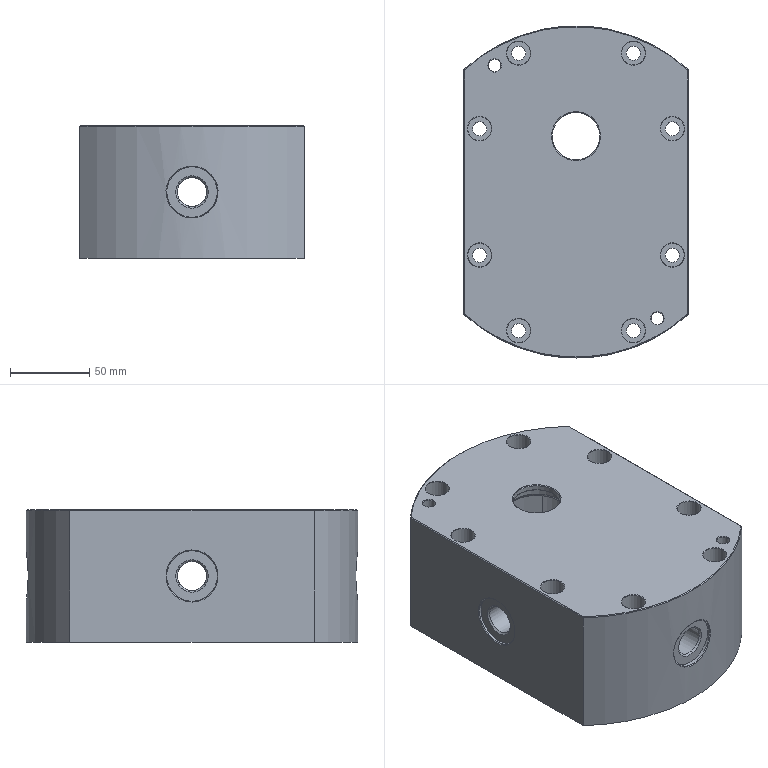NC program | NX | posted with a generic post | part box 142 x 210 x 84 mm
Lines 1 to 686 of 1634:
N10 G17 G21 G94 G90
(HOLE_MILLING_COPY_COPY , TOOL : D10)
N12 T10 M6
N14 G54
N16 G17 G0 G90 X-87.769 Y36.355 B0. C0. S3000 M3
N18 G43 Z30. H10
N20 Z0.5
N22 G94 G3 X-89.019 Y35.105 R1.25 F2200.
N24 X-87.769 Y33.855 R1.25
N26 X-87.769 Y33.855 Z0.28 I0. J2.5
N28 X-87.769 Y33.855 Z0.06 I0. J2.5
N30 X-87.769 Y33.855 Z-0.16 I0. J2.5
N32 X-87.769 Y33.855 Z-0.38 I0. J2.5
N34 X-87.769 Y33.855 Z-0.6 I0. J2.5
N36 X-87.769 Y33.855 Z-0.82 I0. J2.5
N38 X-87.769 Y33.855 Z-1.04 I0. J2.5
N40 X-87.769 Y33.855 Z-1.26 I0. J2.5
N42 X-87.769 Y33.855 Z-1.48 I0. J2.5
N44 X-87.769 Y33.855 Z-1.7 I0. J2.5
N46 X-87.769 Y33.855 Z-1.92 I0. J2.5
N48 X-87.769 Y33.855 Z-2.14 I0. J2.5
N50 X-87.769 Y33.855 Z-2.36 I0. J2.5
N52 X-87.769 Y33.855 Z-2.58 I0. J2.5
N54 X-87.769 Y33.855 Z-2.8 I0. J2.5
N56 X-87.769 Y33.855 Z-3.02 I0. J2.5
N58 X-87.769 Y33.855 Z-3.24 I0. J2.5
N60 X-87.769 Y33.855 Z-3.46 I0. J2.5
N62 X-87.769 Y33.855 Z-3.68 I0. J2.5
N64 X-87.769 Y33.855 Z-3.9 I0. J2.5
N66 X-87.769 Y33.855 Z-4.12 I0. J2.5
N68 X-87.769 Y33.855 Z-4.34 I0. J2.5
N70 X-87.769 Y33.855 Z-4.56 I0. J2.5
N72 X-87.769 Y33.855 Z-4.78 I0. J2.5
N74 X-87.769 Y33.855 Z-5. I0. J2.5
N76 X-87.769 Y33.855 Z-5.22 I0. J2.5
N78 X-87.769 Y33.855 Z-5.44 I0. J2.5
N80 X-87.769 Y33.855 Z-5.66 I0. J2.5
N82 X-87.769 Y33.855 Z-5.88 I0. J2.5
N84 X-87.769 Y33.855 Z-6.1 I0. J2.5
N86 X-87.769 Y33.855 Z-6.32 I0. J2.5
N88 X-87.769 Y33.855 Z-6.54 I0. J2.5
N90 X-87.769 Y33.855 Z-6.76 I0. J2.5
N92 X-87.769 Y33.855 Z-6.98 I0. J2.5
N94 X-87.769 Y33.855 Z-7.2 I0. J2.5
N96 X-87.769 Y33.855 Z-7.42 I0. J2.5
N98 X-87.769 Y33.855 Z-7.64 I0. J2.5
N100 X-87.769 Y33.855 Z-7.86 I0. J2.5
N102 X-87.769 Y33.855 Z-8.08 I0. J2.5
N104 X-87.769 Y33.855 Z-8.3 I0. J2.5
N106 X-87.769 Y33.855 Z-8.52 I0. J2.5
N108 X-87.769 Y33.855 Z-8.74 I0. J2.5
N110 X-87.769 Y33.855 Z-8.96 I0. J2.5
N112 X-87.769 Y33.855 Z-9.18 I0. J2.5
N114 X-87.769 Y33.855 Z-9.4 I0. J2.5
N116 X-87.769 Y33.855 Z-9.62 I0. J2.5
N118 X-87.769 Y33.855 Z-9.84 I0. J2.5
N120 X-87.769 Y33.855 Z-10.06 I0. J2.5
N122 X-87.769 Y33.855 Z-10.28 I0. J2.5
N124 X-87.769 Y33.855 Z-10.5 I0. J2.5
N126 X-87.769 Y33.855 Z-10.72 I0. J2.5
N128 X-87.769 Y33.855 Z-10.94 I0. J2.5
N130 X-87.769 Y33.855 Z-11.16 I0. J2.5
N132 X-87.769 Y33.855 Z-11.38 I0. J2.5
N134 X-87.769 Y33.855 Z-11.6 I0. J2.5
N136 X-87.769 Y33.855 Z-11.82 I0. J2.5
N138 X-87.769 Y33.855 Z-12.04 I0. J2.5
N140 X-87.769 Y33.855 Z-12.26 I0. J2.5
N142 X-87.769 Y33.855 Z-12.48 I0. J2.5
N144 X-87.769 Y33.855 Z-12.7 I0. J2.5
N146 X-87.769 Y33.855 Z-12.92 I0. J2.5
N148 X-87.769 Y33.855 Z-13.14 I0. J2.5
N150 X-87.769 Y33.855 Z-13.36 I0. J2.5
N152 X-87.769 Y33.855 Z-13.58 I0. J2.5
N154 X-87.769 Y33.855 Z-13.8 I0. J2.5
N156 X-87.769 Y33.855 Z-14.02 I0. J2.5
N158 X-87.769 Y33.855 Z-14.24 I0. J2.5
N160 X-87.769 Y33.855 Z-14.46 I0. J2.5
N162 X-87.769 Y33.855 Z-14.68 I0. J2.5
N164 X-87.769 Y33.855 Z-14.9 I0. J2.5
N166 X-87.769 Y33.855 Z-15.12 I0. J2.5
N168 X-87.769 Y33.855 Z-15.34 I0. J2.5
N170 X-87.769 Y33.855 Z-15.56 I0. J2.5
N172 X-87.769 Y33.855 Z-15.78 I0. J2.5
N174 X-87.769 Y33.855 Z-16. I0. J2.5
N176 X-87.769 Y33.855 Z-16.22 I0. J2.5
N178 X-87.769 Y33.855 Z-16.44 I0. J2.5
N180 X-87.769 Y33.855 Z-16.66 I0. J2.5
N182 X-87.769 Y33.855 Z-16.88 I0. J2.5
N184 X-87.769 Y33.855 Z-17.1 I0. J2.5
N186 X-87.769 Y33.855 Z-17.32 I0. J2.5
N188 X-87.769 Y33.855 Z-17.54 I0. J2.5
N190 X-87.769 Y33.855 Z-17.76 I0. J2.5
N192 X-87.769 Y33.855 Z-17.98 I0. J2.5
N194 X-87.769 Y33.855 Z-18.2 I0. J2.5
N196 X-87.769 Y33.855 Z-18.42 I0. J2.5
N198 X-87.769 Y33.855 Z-18.64 I0. J2.5
N200 X-87.769 Y33.855 Z-18.86 I0. J2.5
N202 X-87.769 Y33.855 Z-19.08 I0. J2.5
N204 X-87.769 Y33.855 Z-19.3 I0. J2.5
N206 X-87.769 Y33.855 Z-19.52 I0. J2.5
N208 X-87.769 Y33.855 Z-19.74 I0. J2.5
N210 X-87.769 Y33.855 Z-19.96 I0. J2.5
N212 X-87.769 Y33.855 Z-20.18 I0. J2.5
N214 X-87.769 Y33.855 Z-20.4 I0. J2.5
N216 X-87.769 Y33.855 Z-20.62 I0. J2.5
N218 X-87.769 Y33.855 Z-20.84 I0. J2.5
N220 X-87.769 Y33.855 Z-21.06 I0. J2.5
N222 X-87.769 Y33.855 Z-21.28 I0. J2.5
N224 X-87.769 Y33.855 Z-21.5 I0. J2.5
N226 X-87.769 Y33.855 Z-21.72 I0. J2.5
N228 X-87.769 Y33.855 Z-21.94 I0. J2.5
N230 X-87.769 Y33.855 Z-22.16 I0. J2.5
N232 X-87.769 Y33.855 Z-22.38 I0. J2.5
N234 X-87.769 Y33.855 Z-22.6 I0. J2.5
N236 X-87.769 Y33.855 Z-22.82 I0. J2.5
N238 X-87.769 Y33.855 Z-23.04 I0. J2.5
N240 X-87.769 Y33.855 Z-23.26 I0. J2.5
N242 X-87.769 Y33.855 Z-23.48 I0. J2.5
N244 X-87.769 Y33.855 Z-23.7 I0. J2.5
N246 X-87.769 Y33.855 Z-23.92 I0. J2.5
N248 X-87.769 Y33.855 Z-24.14 I0. J2.5
N250 X-87.769 Y33.855 Z-24.36 I0. J2.5
N252 X-87.769 Y33.855 Z-24.58 I0. J2.5
N254 X-87.769 Y33.855 Z-24.8 I0. J2.5
N256 X-87.769 Y33.855 Z-25.02 I0. J2.5
N258 X-87.769 Y33.855 Z-25.24 I0. J2.5
N260 X-87.769 Y33.855 Z-25.46 I0. J2.5
N262 X-87.769 Y33.855 Z-25.68 I0. J2.5
N264 X-87.769 Y33.855 Z-25.9 I0. J2.5
N266 X-87.769 Y33.855 Z-26.12 I0. J2.5
N268 X-87.769 Y33.855 Z-26.34 I0. J2.5
N270 X-87.769 Y33.855 Z-26.56 I0. J2.5
N272 X-87.769 Y33.855 Z-26.78 I0. J2.5
N274 X-87.769 Y33.855 Z-27. I0. J2.5
N276 X-87.769 Y33.855 Z-27.22 I0. J2.5
N278 X-87.769 Y33.855 Z-27.44 I0. J2.5
N280 X-87.769 Y33.855 Z-27.66 I0. J2.5
N282 X-87.769 Y33.855 Z-27.88 I0. J2.5
N284 X-87.769 Y33.855 Z-28.1 I0. J2.5
N286 X-87.769 Y33.855 Z-28.32 I0. J2.5
N288 X-87.769 Y33.855 Z-28.54 I0. J2.5
N290 X-87.769 Y33.855 Z-28.76 I0. J2.5
N292 X-87.769 Y33.855 Z-28.98 I0. J2.5
N294 X-87.769 Y33.855 Z-29.2 I0. J2.5
N296 X-87.769 Y33.855 Z-29.42 I0. J2.5
N298 X-87.769 Y33.855 Z-29.64 I0. J2.5
N300 X-87.769 Y33.855 Z-29.86 I0. J2.5
N302 X-87.769 Y33.855 Z-30.08 I0. J2.5
N304 X-87.769 Y33.855 Z-30.3 I0. J2.5
N306 X-87.769 Y33.855 Z-30.52 I0. J2.5
N308 X-87.769 Y33.855 Z-30.74 I0. J2.5
N310 X-87.769 Y33.855 Z-30.96 I0. J2.5
N312 X-87.769 Y33.855 Z-31.18 I0. J2.5
N314 X-87.769 Y33.855 Z-31.4 I0. J2.5
N316 X-87.769 Y33.855 Z-31.62 I0. J2.5
N318 X-87.769 Y33.855 Z-31.84 I0. J2.5
N320 X-87.769 Y33.855 Z-32.06 I0. J2.5
N322 X-87.769 Y33.855 Z-32.28 I0. J2.5
N324 X-87.769 Y33.855 Z-32.5 I0. J2.5
N326 X-87.769 Y33.855 Z-32.72 I0. J2.5
N328 X-87.769 Y33.855 Z-32.94 I0. J2.5
N330 X-87.769 Y33.855 Z-33.16 I0. J2.5
N332 X-87.769 Y33.855 Z-33.38 I0. J2.5
N334 X-87.769 Y33.855 Z-33.6 I0. J2.5
N336 X-87.769 Y33.855 Z-33.82 I0. J2.5
N338 X-87.769 Y33.855 Z-34.04 I0. J2.5
N340 X-87.769 Y33.855 Z-34.26 I0. J2.5
N342 X-87.769 Y33.855 Z-34.48 I0. J2.5
N344 X-87.769 Y33.855 Z-34.7 I0. J2.5
N346 X-87.769 Y33.855 Z-34.92 I0. J2.5
N348 X-85.879 Y37.992 Z-35. R2.5
N350 X-89.406 Y38.244 R2.5
N352 X-85.879 Y37.992 R-2.5
N354 X-87.642 Y38.118 R1.25
N356 X-87.769 Y36.355 R1.25
N358 G0 Z30.
N360 X-40. Y61.
N362 Z0.5
N364 G3 X-41.25 Y59.75 R1.25
N366 X-40. Y58.5 R1.25
N368 X-40. Y58.5 Z0.28 I0. J2.5
N370 X-40. Y58.5 Z0.06 I0. J2.5
N372 X-40. Y58.5 Z-0.16 I0. J2.5
N374 X-40. Y58.5 Z-0.38 I0. J2.5
N376 X-40. Y58.5 Z-0.6 I0. J2.5
N378 X-40. Y58.5 Z-0.82 I0. J2.5
N380 X-40. Y58.5 Z-1.04 I0. J2.5
N382 X-40. Y58.5 Z-1.26 I0. J2.5
N384 X-40. Y58.5 Z-1.48 I0. J2.5
N386 X-40. Y58.5 Z-1.7 I0. J2.5
N388 X-40. Y58.5 Z-1.92 I0. J2.5
N390 X-40. Y58.5 Z-2.14 I0. J2.5
N392 X-40. Y58.5 Z-2.36 I0. J2.5
N394 X-40. Y58.5 Z-2.58 I0. J2.5
N396 X-40. Y58.5 Z-2.8 I0. J2.5
N398 X-40. Y58.5 Z-3.02 I0. J2.5
N400 X-40. Y58.5 Z-3.24 I0. J2.5
N402 X-40. Y58.5 Z-3.46 I0. J2.5
N404 X-40. Y58.5 Z-3.68 I0. J2.5
N406 X-40. Y58.5 Z-3.9 I0. J2.5
N408 X-40. Y58.5 Z-4.12 I0. J2.5
N410 X-40. Y58.5 Z-4.34 I0. J2.5
N412 X-40. Y58.5 Z-4.56 I0. J2.5
N414 X-40. Y58.5 Z-4.78 I0. J2.5
N416 X-40. Y58.5 Z-5. I0. J2.5
N418 X-40. Y58.5 Z-5.22 I0. J2.5
N420 X-40. Y58.5 Z-5.44 I0. J2.5
N422 X-40. Y58.5 Z-5.66 I0. J2.5
N424 X-40. Y58.5 Z-5.88 I0. J2.5
N426 X-40. Y58.5 Z-6.1 I0. J2.5
N428 X-40. Y58.5 Z-6.32 I0. J2.5
N430 X-40. Y58.5 Z-6.54 I0. J2.5
N432 X-40. Y58.5 Z-6.76 I0. J2.5
N434 X-40. Y58.5 Z-6.98 I0. J2.5
N436 X-40. Y58.5 Z-7.2 I0. J2.5
N438 X-40. Y58.5 Z-7.42 I0. J2.5
N440 X-40. Y58.5 Z-7.64 I0. J2.5
N442 X-40. Y58.5 Z-7.86 I0. J2.5
N444 X-40. Y58.5 Z-8.08 I0. J2.5
N446 X-40. Y58.5 Z-8.3 I0. J2.5
N448 X-40. Y58.5 Z-8.52 I0. J2.5
N450 X-40. Y58.5 Z-8.74 I0. J2.5
N452 X-40. Y58.5 Z-8.96 I0. J2.5
N454 X-40. Y58.5 Z-9.18 I0. J2.5
N456 X-40. Y58.5 Z-9.4 I0. J2.5
N458 X-40. Y58.5 Z-9.62 I0. J2.5
N460 X-40. Y58.5 Z-9.84 I0. J2.5
N462 X-40. Y58.5 Z-10.06 I0. J2.5
N464 X-40. Y58.5 Z-10.28 I0. J2.5
N466 X-40. Y58.5 Z-10.5 I0. J2.5
N468 X-40. Y58.5 Z-10.72 I0. J2.5
N470 X-40. Y58.5 Z-10.94 I0. J2.5
N472 X-40. Y58.5 Z-11.16 I0. J2.5
N474 X-40. Y58.5 Z-11.38 I0. J2.5
N476 X-40. Y58.5 Z-11.6 I0. J2.5
N478 X-40. Y58.5 Z-11.82 I0. J2.5
N480 X-40. Y58.5 Z-12.04 I0. J2.5
N482 X-40. Y58.5 Z-12.26 I0. J2.5
N484 X-40. Y58.5 Z-12.48 I0. J2.5
N486 X-40. Y58.5 Z-12.7 I0. J2.5
N488 X-40. Y58.5 Z-12.92 I0. J2.5
N490 X-40. Y58.5 Z-13.14 I0. J2.5
N492 X-40. Y58.5 Z-13.36 I0. J2.5
N494 X-40. Y58.5 Z-13.58 I0. J2.5
N496 X-40. Y58.5 Z-13.8 I0. J2.5
N498 X-40. Y58.5 Z-14.02 I0. J2.5
N500 X-40. Y58.5 Z-14.24 I0. J2.5
N502 X-40. Y58.5 Z-14.46 I0. J2.5
N504 X-40. Y58.5 Z-14.68 I0. J2.5
N506 X-40. Y58.5 Z-14.9 I0. J2.5
N508 X-40. Y58.5 Z-15.12 I0. J2.5
N510 X-40. Y58.5 Z-15.34 I0. J2.5
N512 X-40. Y58.5 Z-15.56 I0. J2.5
N514 X-40. Y58.5 Z-15.78 I0. J2.5
N516 X-40. Y58.5 Z-16. I0. J2.5
N518 X-40. Y58.5 Z-16.22 I0. J2.5
N520 X-40. Y58.5 Z-16.44 I0. J2.5
N522 X-40. Y58.5 Z-16.66 I0. J2.5
N524 X-40. Y58.5 Z-16.88 I0. J2.5
N526 X-40. Y58.5 Z-17.1 I0. J2.5
N528 X-40. Y58.5 Z-17.32 I0. J2.5
N530 X-40. Y58.5 Z-17.54 I0. J2.5
N532 X-40. Y58.5 Z-17.76 I0. J2.5
N534 X-40. Y58.5 Z-17.98 I0. J2.5
N536 X-40. Y58.5 Z-18.2 I0. J2.5
N538 X-40. Y58.5 Z-18.42 I0. J2.5
N540 X-40. Y58.5 Z-18.64 I0. J2.5
N542 X-40. Y58.5 Z-18.86 I0. J2.5
N544 X-40. Y58.5 Z-19.08 I0. J2.5
N546 X-40. Y58.5 Z-19.3 I0. J2.5
N548 X-40. Y58.5 Z-19.52 I0. J2.5
N550 X-40. Y58.5 Z-19.74 I0. J2.5
N552 X-40. Y58.5 Z-19.96 I0. J2.5
N554 X-40. Y58.5 Z-20.18 I0. J2.5
N556 X-40. Y58.5 Z-20.4 I0. J2.5
N558 X-40. Y58.5 Z-20.62 I0. J2.5
N560 X-40. Y58.5 Z-20.84 I0. J2.5
N562 X-40. Y58.5 Z-21.06 I0. J2.5
N564 X-40. Y58.5 Z-21.28 I0. J2.5
N566 X-40. Y58.5 Z-21.5 I0. J2.5
N568 X-40. Y58.5 Z-21.72 I0. J2.5
N570 X-40. Y58.5 Z-21.94 I0. J2.5
N572 X-40. Y58.5 Z-22.16 I0. J2.5
N574 X-40. Y58.5 Z-22.38 I0. J2.5
N576 X-40. Y58.5 Z-22.6 I0. J2.5
N578 X-40. Y58.5 Z-22.82 I0. J2.5
N580 X-40. Y58.5 Z-23.04 I0. J2.5
N582 X-40. Y58.5 Z-23.26 I0. J2.5
N584 X-40. Y58.5 Z-23.48 I0. J2.5
N586 X-40. Y58.5 Z-23.7 I0. J2.5
N588 X-40. Y58.5 Z-23.92 I0. J2.5
N590 X-40. Y58.5 Z-24.14 I0. J2.5
N592 X-40. Y58.5 Z-24.36 I0. J2.5
N594 X-40. Y58.5 Z-24.58 I0. J2.5
N596 X-40. Y58.5 Z-24.8 I0. J2.5
N598 X-40. Y58.5 Z-25.02 I0. J2.5
N600 X-40. Y58.5 Z-25.24 I0. J2.5
N602 X-40. Y58.5 Z-25.46 I0. J2.5
N604 X-40. Y58.5 Z-25.68 I0. J2.5
N606 X-40. Y58.5 Z-25.9 I0. J2.5
N608 X-40. Y58.5 Z-26.12 I0. J2.5
N610 X-40. Y58.5 Z-26.34 I0. J2.5
N612 X-40. Y58.5 Z-26.56 I0. J2.5
N614 X-40. Y58.5 Z-26.78 I0. J2.5
N616 X-40. Y58.5 Z-27. I0. J2.5
N618 X-40. Y58.5 Z-27.22 I0. J2.5
N620 X-40. Y58.5 Z-27.44 I0. J2.5
N622 X-40. Y58.5 Z-27.66 I0. J2.5
N624 X-40. Y58.5 Z-27.88 I0. J2.5
N626 X-40. Y58.5 Z-28.1 I0. J2.5
N628 X-40. Y58.5 Z-28.32 I0. J2.5
N630 X-40. Y58.5 Z-28.54 I0. J2.5
N632 X-40. Y58.5 Z-28.76 I0. J2.5
N634 X-40. Y58.5 Z-28.98 I0. J2.5
N636 X-40. Y58.5 Z-29.2 I0. J2.5
N638 X-40. Y58.5 Z-29.42 I0. J2.5
N640 X-40. Y58.5 Z-29.64 I0. J2.5
N642 X-40. Y58.5 Z-29.86 I0. J2.5
N644 X-40. Y58.5 Z-30.08 I0. J2.5
N646 X-40. Y58.5 Z-30.3 I0. J2.5
N648 X-40. Y58.5 Z-30.52 I0. J2.5
N650 X-40. Y58.5 Z-30.74 I0. J2.5
N652 X-40. Y58.5 Z-30.96 I0. J2.5
N654 X-40. Y58.5 Z-31.18 I0. J2.5
N656 X-40. Y58.5 Z-31.4 I0. J2.5
N658 X-40. Y58.5 Z-31.62 I0. J2.5
N660 X-40. Y58.5 Z-31.84 I0. J2.5
N662 X-40. Y58.5 Z-32.06 I0. J2.5
N664 X-40. Y58.5 Z-32.28 I0. J2.5
N666 X-40. Y58.5 Z-32.5 I0. J2.5
N668 X-40. Y58.5 Z-32.72 I0. J2.5
N670 X-40. Y58.5 Z-32.94 I0. J2.5
N672 X-40. Y58.5 Z-33.16 I0. J2.5
N674 X-40. Y58.5 Z-33.38 I0. J2.5
N676 X-40. Y58.5 Z-33.6 I0. J2.5
N678 X-40. Y58.5 Z-33.82 I0. J2.5
N680 X-40. Y58.5 Z-34.04 I0. J2.5
N682 X-40. Y58.5 Z-34.26 I0. J2.5
N684 X-40. Y58.5 Z-34.48 I0. J2.5
N686 X-40. Y58.5 Z-34.7 I0. J2.5
N688 X-40. Y58.5 Z-34.92 I0. J2.5
N690 X-38.111 Y62.637 Z-35. R2.5
N692 X-41.637 Y62.889 R2.5
N694 X-38.111 Y62.637 R-2.5
N696 X-39.874 Y62.763 R1.25
N698 X-40. Y61. R1.25
N700 G0 Z30.
N702 X40.
N704 Z0.5
N706 G3 X38.75 Y59.75 R1.25
N708 X40. Y58.5 R1.25
N710 X40. Y58.5 Z0.28 I0. J2.5
N712 X40. Y58.5 Z0.06 I0. J2.5
N714 X40. Y58.5 Z-0.16 I0. J2.5
N716 X40. Y58.5 Z-0.38 I0. J2.5
N718 X40. Y58.5 Z-0.6 I0. J2.5
N720 X40. Y58.5 Z-0.82 I0. J2.5
N722 X40. Y58.5 Z-1.04 I0. J2.5
N724 X40. Y58.5 Z-1.26 I0. J2.5
N726 X40. Y58.5 Z-1.48 I0. J2.5
N728 X40. Y58.5 Z-1.7 I0. J2.5
N730 X40. Y58.5 Z-1.92 I0. J2.5
N732 X40. Y58.5 Z-2.14 I0. J2.5
N734 X40. Y58.5 Z-2.36 I0. J2.5
N736 X40. Y58.5 Z-2.58 I0. J2.5
N738 X40. Y58.5 Z-2.8 I0. J2.5
N740 X40. Y58.5 Z-3.02 I0. J2.5
N742 X40. Y58.5 Z-3.24 I0. J2.5
N744 X40. Y58.5 Z-3.46 I0. J2.5
N746 X40. Y58.5 Z-3.68 I0. J2.5
N748 X40. Y58.5 Z-3.9 I0. J2.5
N750 X40. Y58.5 Z-4.12 I0. J2.5
N752 X40. Y58.5 Z-4.34 I0. J2.5
N754 X40. Y58.5 Z-4.56 I0. J2.5
N756 X40. Y58.5 Z-4.78 I0. J2.5
N758 X40. Y58.5 Z-5. I0. J2.5
N760 X40. Y58.5 Z-5.22 I0. J2.5
N762 X40. Y58.5 Z-5.44 I0. J2.5
N764 X40. Y58.5 Z-5.66 I0. J2.5
N766 X40. Y58.5 Z-5.88 I0. J2.5
N768 X40. Y58.5 Z-6.1 I0. J2.5
N770 X40. Y58.5 Z-6.32 I0. J2.5
N772 X40. Y58.5 Z-6.54 I0. J2.5
N774 X40. Y58.5 Z-6.76 I0. J2.5
N776 X40. Y58.5 Z-6.98 I0. J2.5
N778 X40. Y58.5 Z-7.2 I0. J2.5
N780 X40. Y58.5 Z-7.42 I0. J2.5
N782 X40. Y58.5 Z-7.64 I0. J2.5
N784 X40. Y58.5 Z-7.86 I0. J2.5
N786 X40. Y58.5 Z-8.08 I0. J2.5
N788 X40. Y58.5 Z-8.3 I0. J2.5
N790 X40. Y58.5 Z-8.52 I0. J2.5
N792 X40. Y58.5 Z-8.74 I0. J2.5
N794 X40. Y58.5 Z-8.96 I0. J2.5
N796 X40. Y58.5 Z-9.18 I0. J2.5
N798 X40. Y58.5 Z-9.4 I0. J2.5
N800 X40. Y58.5 Z-9.62 I0. J2.5
N802 X40. Y58.5 Z-9.84 I0. J2.5
N804 X40. Y58.5 Z-10.06 I0. J2.5
N806 X40. Y58.5 Z-10.28 I0. J2.5
N808 X40. Y58.5 Z-10.5 I0. J2.5
N810 X40. Y58.5 Z-10.72 I0. J2.5
N812 X40. Y58.5 Z-10.94 I0. J2.5
N814 X40. Y58.5 Z-11.16 I0. J2.5
N816 X40. Y58.5 Z-11.38 I0. J2.5
N818 X40. Y58.5 Z-11.6 I0. J2.5
N820 X40. Y58.5 Z-11.82 I0. J2.5
N822 X40. Y58.5 Z-12.04 I0. J2.5
N824 X40. Y58.5 Z-12.26 I0. J2.5
N826 X40. Y58.5 Z-12.48 I0. J2.5
N828 X40. Y58.5 Z-12.7 I0. J2.5
N830 X40. Y58.5 Z-12.92 I0. J2.5
N832 X40. Y58.5 Z-13.14 I0. J2.5
N834 X40. Y58.5 Z-13.36 I0. J2.5
N836 X40. Y58.5 Z-13.58 I0. J2.5
N838 X40. Y58.5 Z-13.8 I0. J2.5
N840 X40. Y58.5 Z-14.02 I0. J2.5
N842 X40. Y58.5 Z-14.24 I0. J2.5
N844 X40. Y58.5 Z-14.46 I0. J2.5
N846 X40. Y58.5 Z-14.68 I0. J2.5
N848 X40. Y58.5 Z-14.9 I0. J2.5
N850 X40. Y58.5 Z-15.12 I0. J2.5
N852 X40. Y58.5 Z-15.34 I0. J2.5
N854 X40. Y58.5 Z-15.56 I0. J2.5
N856 X40. Y58.5 Z-15.78 I0. J2.5
N858 X40. Y58.5 Z-16. I0. J2.5
N860 X40. Y58.5 Z-16.22 I0. J2.5
N862 X40. Y58.5 Z-16.44 I0. J2.5
N864 X40. Y58.5 Z-16.66 I0. J2.5
N866 X40. Y58.5 Z-16.88 I0. J2.5
N868 X40. Y58.5 Z-17.1 I0. J2.5
N870 X40. Y58.5 Z-17.32 I0. J2.5
N872 X40. Y58.5 Z-17.54 I0. J2.5
N874 X40. Y58.5 Z-17.76 I0. J2.5
N876 X40. Y58.5 Z-17.98 I0. J2.5
N878 X40. Y58.5 Z-18.2 I0. J2.5
N880 X40. Y58.5 Z-18.42 I0. J2.5
N882 X40. Y58.5 Z-18.64 I0. J2.5
N884 X40. Y58.5 Z-18.86 I0. J2.5
N886 X40. Y58.5 Z-19.08 I0. J2.5
N888 X40. Y58.5 Z-19.3 I0. J2.5
N890 X40. Y58.5 Z-19.52 I0. J2.5
N892 X40. Y58.5 Z-19.74 I0. J2.5
N894 X40. Y58.5 Z-19.96 I0. J2.5
N896 X40. Y58.5 Z-20.18 I0. J2.5
N898 X40. Y58.5 Z-20.4 I0. J2.5
N900 X40. Y58.5 Z-20.62 I0. J2.5
N902 X40. Y58.5 Z-20.84 I0. J2.5
N904 X40. Y58.5 Z-21.06 I0. J2.5
N906 X40. Y58.5 Z-21.28 I0. J2.5
N908 X40. Y58.5 Z-21.5 I0. J2.5
N910 X40. Y58.5 Z-21.72 I0. J2.5
N912 X40. Y58.5 Z-21.94 I0. J2.5
N914 X40. Y58.5 Z-22.16 I0. J2.5
N916 X40. Y58.5 Z-22.38 I0. J2.5
N918 X40. Y58.5 Z-22.6 I0. J2.5
N920 X40. Y58.5 Z-22.82 I0. J2.5
N922 X40. Y58.5 Z-23.04 I0. J2.5
N924 X40. Y58.5 Z-23.26 I0. J2.5
N926 X40. Y58.5 Z-23.48 I0. J2.5
N928 X40. Y58.5 Z-23.7 I0. J2.5
N930 X40. Y58.5 Z-23.92 I0. J2.5
N932 X40. Y58.5 Z-24.14 I0. J2.5
N934 X40. Y58.5 Z-24.36 I0. J2.5
N936 X40. Y58.5 Z-24.58 I0. J2.5
N938 X40. Y58.5 Z-24.8 I0. J2.5
N940 X40. Y58.5 Z-25.02 I0. J2.5
N942 X40. Y58.5 Z-25.24 I0. J2.5
N944 X40. Y58.5 Z-25.46 I0. J2.5
N946 X40. Y58.5 Z-25.68 I0. J2.5
N948 X40. Y58.5 Z-25.9 I0. J2.5
N950 X40. Y58.5 Z-26.12 I0. J2.5
N952 X40. Y58.5 Z-26.34 I0. J2.5
N954 X40. Y58.5 Z-26.56 I0. J2.5
N956 X40. Y58.5 Z-26.78 I0. J2.5
N958 X40. Y58.5 Z-27. I0. J2.5
N960 X40. Y58.5 Z-27.22 I0. J2.5
N962 X40. Y58.5 Z-27.44 I0. J2.5
N964 X40. Y58.5 Z-27.66 I0. J2.5
N966 X40. Y58.5 Z-27.88 I0. J2.5
N968 X40. Y58.5 Z-28.1 I0. J2.5
N970 X40. Y58.5 Z-28.32 I0. J2.5
N972 X40. Y58.5 Z-28.54 I0. J2.5
N974 X40. Y58.5 Z-28.76 I0. J2.5
N976 X40. Y58.5 Z-28.98 I0. J2.5
N978 X40. Y58.5 Z-29.2 I0. J2.5
N980 X40. Y58.5 Z-29.42 I0. J2.5
N982 X40. Y58.5 Z-29.64 I0. J2.5
N984 X40. Y58.5 Z-29.86 I0. J2.5
N986 X40. Y58.5 Z-30.08 I0. J2.5
N988 X40. Y58.5 Z-30.3 I0. J2.5
N990 X40. Y58.5 Z-30.52 I0. J2.5
N992 X40. Y58.5 Z-30.74 I0. J2.5
N994 X40. Y58.5 Z-30.96 I0. J2.5
N996 X40. Y58.5 Z-31.18 I0. J2.5
N998 X40. Y58.5 Z-31.4 I0. J2.5
N1000 X40. Y58.5 Z-31.62 I0. J2.5
N1002 X40. Y58.5 Z-31.84 I0. J2.5
N1004 X40. Y58.5 Z-32.06 I0. J2.5
N1006 X40. Y58.5 Z-32.28 I0. J2.5
N1008 X40. Y58.5 Z-32.5 I0. J2.5
N1010 X40. Y58.5 Z-32.72 I0. J2.5
N1012 X40. Y58.5 Z-32.94 I0. J2.5
N1014 X40. Y58.5 Z-33.16 I0. J2.5
N1016 X40. Y58.5 Z-33.38 I0. J2.5
N1018 X40. Y58.5 Z-33.6 I0. J2.5
N1020 X40. Y58.5 Z-33.82 I0. J2.5
N1022 X40. Y58.5 Z-34.04 I0. J2.5
N1024 X40. Y58.5 Z-34.26 I0. J2.5
N1026 X40. Y58.5 Z-34.48 I0. J2.5
N1028 X40. Y58.5 Z-34.7 I0. J2.5
N1030 X40. Y58.5 Z-34.92 I0. J2.5
N1032 X41.889 Y62.637 Z-35. R2.5
N1034 X38.363 Y62.889 R2.5
N1036 X41.889 Y62.637 R-2.5
N1038 X40.126 Y62.763 R1.25
N1040 X40. Y61. R1.25
N1042 G0 Z30.
N1044 X87.769 Y36.355
N1046 Z0.5
N1048 G3 X86.519 Y35.105 R1.25
N1050 X87.769 Y33.855 R1.25
N1052 X87.769 Y33.855 Z0.28 I0. J2.5
N1054 X87.769 Y33.855 Z0.06 I0. J2.5
N1056 X87.769 Y33.855 Z-0.16 I0. J2.5
N1058 X87.769 Y33.855 Z-0.38 I0. J2.5
N1060 X87.769 Y33.855 Z-0.6 I0. J2.5
N1062 X87.769 Y33.855 Z-0.82 I0. J2.5
N1064 X87.769 Y33.855 Z-1.04 I0. J2.5
N1066 X87.769 Y33.855 Z-1.26 I0. J2.5
N1068 X87.769 Y33.855 Z-1.48 I0. J2.5
N1070 X87.769 Y33.855 Z-1.7 I0. J2.5
N1072 X87.769 Y33.855 Z-1.92 I0. J2.5
N1074 X87.769 Y33.855 Z-2.14 I0. J2.5
N1076 X87.769 Y33.855 Z-2.36 I0. J2.5
N1078 X87.769 Y33.855 Z-2.58 I0. J2.5
N1080 X87.769 Y33.855 Z-2.8 I0. J2.5
N1082 X87.769 Y33.855 Z-3.02 I0. J2.5
N1084 X87.769 Y33.855 Z-3.24 I0. J2.5
N1086 X87.769 Y33.855 Z-3.46 I0. J2.5
N1088 X87.769 Y33.855 Z-3.68 I0. J2.5
N1090 X87.769 Y33.855 Z-3.9 I0. J2.5
N1092 X87.769 Y33.855 Z-4.12 I0. J2.5
N1094 X87.769 Y33.855 Z-4.34 I0. J2.5
N1096 X87.769 Y33.855 Z-4.56 I0. J2.5
N1098 X87.769 Y33.855 Z-4.78 I0. J2.5
N1100 X87.769 Y33.855 Z-5. I0. J2.5
N1102 X87.769 Y33.855 Z-5.22 I0. J2.5
N1104 X87.769 Y33.855 Z-5.44 I0. J2.5
N1106 X87.769 Y33.855 Z-5.66 I0. J2.5
N1108 X87.769 Y33.855 Z-5.88 I0. J2.5
N1110 X87.769 Y33.855 Z-6.1 I0. J2.5
N1112 X87.769 Y33.855 Z-6.32 I0. J2.5
N1114 X87.769 Y33.855 Z-6.54 I0. J2.5
N1116 X87.769 Y33.855 Z-6.76 I0. J2.5
N1118 X87.769 Y33.855 Z-6.98 I0. J2.5
N1120 X87.769 Y33.855 Z-7.2 I0. J2.5
N1122 X87.769 Y33.855 Z-7.42 I0. J2.5
N1124 X87.769 Y33.855 Z-7.64 I0. J2.5
N1126 X87.769 Y33.855 Z-7.86 I0. J2.5
N1128 X87.769 Y33.855 Z-8.08 I0. J2.5
N1130 X87.769 Y33.855 Z-8.3 I0. J2.5
N1132 X87.769 Y33.855 Z-8.52 I0. J2.5
N1134 X87.769 Y33.855 Z-8.74 I0. J2.5
N1136 X87.769 Y33.855 Z-8.96 I0. J2.5
N1138 X87.769 Y33.855 Z-9.18 I0. J2.5
N1140 X87.769 Y33.855 Z-9.4 I0. J2.5
N1142 X87.769 Y33.855 Z-9.62 I0. J2.5
N1144 X87.769 Y33.855 Z-9.84 I0. J2.5
N1146 X87.769 Y33.855 Z-10.06 I0. J2.5
N1148 X87.769 Y33.855 Z-10.28 I0. J2.5
N1150 X87.769 Y33.855 Z-10.5 I0. J2.5
N1152 X87.769 Y33.855 Z-10.72 I0. J2.5
N1154 X87.769 Y33.855 Z-10.94 I0. J2.5
N1156 X87.769 Y33.855 Z-11.16 I0. J2.5
N1158 X87.769 Y33.855 Z-11.38 I0. J2.5
N1160 X87.769 Y33.855 Z-11.6 I0. J2.5
N1162 X87.769 Y33.855 Z-11.82 I0. J2.5
N1164 X87.769 Y33.855 Z-12.04 I0. J2.5
N1166 X87.769 Y33.855 Z-12.26 I0. J2.5
N1168 X87.769 Y33.855 Z-12.48 I0. J2.5
N1170 X87.769 Y33.855 Z-12.7 I0. J2.5
N1172 X87.769 Y33.855 Z-12.92 I0. J2.5
N1174 X87.769 Y33.855 Z-13.14 I0. J2.5
N1176 X87.769 Y33.855 Z-13.36 I0. J2.5
N1178 X87.769 Y33.855 Z-13.58 I0. J2.5
N1180 X87.769 Y33.855 Z-13.8 I0. J2.5
N1182 X87.769 Y33.855 Z-14.02 I0. J2.5
N1184 X87.769 Y33.855 Z-14.24 I0. J2.5
N1186 X87.769 Y33.855 Z-14.46 I0. J2.5
N1188 X87.769 Y33.855 Z-14.68 I0. J2.5
N1190 X87.769 Y33.855 Z-14.9 I0. J2.5
N1192 X87.769 Y33.855 Z-15.12 I0. J2.5
N1194 X87.769 Y33.855 Z-15.34 I0. J2.5
N1196 X87.769 Y33.855 Z-15.56 I0. J2.5
N1198 X87.769 Y33.855 Z-15.78 I0. J2.5
N1200 X87.769 Y33.855 Z-16. I0. J2.5
N1202 X87.769 Y33.855 Z-16.22 I0. J2.5
N1204 X87.769 Y33.855 Z-16.44 I0. J2.5
N1206 X87.769 Y33.855 Z-16.66 I0. J2.5
N1208 X87.769 Y33.855 Z-16.88 I0. J2.5
N1210 X87.769 Y33.855 Z-17.1 I0. J2.5
N1212 X87.769 Y33.855 Z-17.32 I0. J2.5
N1214 X87.769 Y33.855 Z-17.54 I0. J2.5
N1216 X87.769 Y33.855 Z-17.76 I0. J2.5
N1218 X87.769 Y33.855 Z-17.98 I0. J2.5
N1220 X87.769 Y33.855 Z-18.2 I0. J2.5
N1222 X87.769 Y33.855 Z-18.42 I0. J2.5
N1224 X87.769 Y33.855 Z-18.64 I0. J2.5
N1226 X87.769 Y33.855 Z-18.86 I0. J2.5
N1228 X87.769 Y33.855 Z-19.08 I0. J2.5
N1230 X87.769 Y33.855 Z-19.3 I0. J2.5
N1232 X87.769 Y33.855 Z-19.52 I0. J2.5
N1234 X87.769 Y33.855 Z-19.74 I0. J2.5
N1236 X87.769 Y33.855 Z-19.96 I0. J2.5
N1238 X87.769 Y33.855 Z-20.18 I0. J2.5
N1240 X87.769 Y33.855 Z-20.4 I0. J2.5
N1242 X87.769 Y33.855 Z-20.62 I0. J2.5
N1244 X87.769 Y33.855 Z-20.84 I0. J2.5
N1246 X87.769 Y33.855 Z-21.06 I0. J2.5
N1248 X87.769 Y33.855 Z-21.28 I0. J2.5
N1250 X87.769 Y33.855 Z-21.5 I0. J2.5
N1252 X87.769 Y33.855 Z-21.72 I0. J2.5
N1254 X87.769 Y33.855 Z-21.94 I0. J2.5
N1256 X87.769 Y33.855 Z-22.16 I0. J2.5
N1258 X87.769 Y33.855 Z-22.38 I0. J2.5
N1260 X87.769 Y33.855 Z-22.6 I0. J2.5
N1262 X87.769 Y33.855 Z-22.82 I0. J2.5
N1264 X87.769 Y33.855 Z-23.04 I0. J2.5
N1266 X87.769 Y33.855 Z-23.26 I0. J2.5
N1268 X87.769 Y33.855 Z-23.48 I0. J2.5
N1270 X87.769 Y33.855 Z-23.7 I0. J2.5
N1272 X87.769 Y33.855 Z-23.92 I0. J2.5
N1274 X87.769 Y33.855 Z-24.14 I0. J2.5
N1276 X87.769 Y33.855 Z-24.36 I0. J2.5
N1278 X87.769 Y33.855 Z-24.58 I0. J2.5
N1280 X87.769 Y33.855 Z-24.8 I0. J2.5
N1282 X87.769 Y33.855 Z-25.02 I0. J2.5
N1284 X87.769 Y33.855 Z-25.24 I0. J2.5
N1286 X87.769 Y33.855 Z-25.46 I0. J2.5
N1288 X87.769 Y33.855 Z-25.68 I0. J2.5
N1290 X87.769 Y33.855 Z-25.9 I0. J2.5
N1292 X87.769 Y33.855 Z-26.12 I0. J2.5
N1294 X87.769 Y33.855 Z-26.34 I0. J2.5
N1296 X87.769 Y33.855 Z-26.56 I0. J2.5
N1298 X87.769 Y33.855 Z-26.78 I0. J2.5
N1300 X87.769 Y33.855 Z-27. I0. J2.5
N1302 X87.769 Y33.855 Z-27.22 I0. J2.5
N1304 X87.769 Y33.855 Z-27.44 I0. J2.5
N1306 X87.769 Y33.855 Z-27.66 I0. J2.5
N1308 X87.769 Y33.855 Z-27.88 I0. J2.5
N1310 X87.769 Y33.855 Z-28.1 I0. J2.5
N1312 X87.769 Y33.855 Z-28.32 I0. J2.5
N1314 X87.769 Y33.855 Z-28.54 I0. J2.5
N1316 X87.769 Y33.855 Z-28.76 I0. J2.5
N1318 X87.769 Y33.855 Z-28.98 I0. J2.5
N1320 X87.769 Y33.855 Z-29.2 I0. J2.5
N1322 X87.769 Y33.855 Z-29.42 I0. J2.5
N1324 X87.769 Y33.855 Z-29.64 I0. J2.5
N1326 X87.769 Y33.855 Z-29.86 I0. J2.5
N1328 X87.769 Y33.855 Z-30.08 I0. J2.5
N1330 X87.769 Y33.855 Z-30.3 I0. J2.5
N1332 X87.769 Y33.855 Z-30.52 I0. J2.5
N1334 X87.769 Y33.855 Z-30.74 I0. J2.5
N1336 X87.769 Y33.855 Z-30.96 I0. J2.5
N1338 X87.769 Y33.855 Z-31.18 I0. J2.5
N1340 X87.769 Y33.855 Z-31.4 I0. J2.5
N1342 X87.769 Y33.855 Z-31.62 I0. J2.5
N1344 X87.769 Y33.855 Z-31.84 I0. J2.5
N1346 X87.769 Y33.855 Z-32.06 I0. J2.5
N1348 X87.769 Y33.855 Z-32.28 I0. J2.5
N1350 X87.769 Y33.855 Z-32.5 I0. J2.5
N1352 X87.769 Y33.855 Z-32.72 I0. J2.5
N1354 X87.769 Y33.855 Z-32.94 I0. J2.5
N1356 X87.769 Y33.855 Z-33.16 I0. J2.5
N1358 X87.769 Y33.855 Z-33.38 I0. J2.5
N1360 X87.769 Y33.855 Z-33.6 I0. J2.5
N1362 X87.769 Y33.855 Z-33.82 I0. J2.5
N1364 X87.769 Y33.855 Z-34.04 I0. J2.5
N1366 X87.769 Y33.855 Z-34.26 I0. J2.5
N1368 X87.769 Y33.855 Z-34.48 I0. J2.5
N1370 X87.769 Y33.855 Z-34.7 I0. J2.5